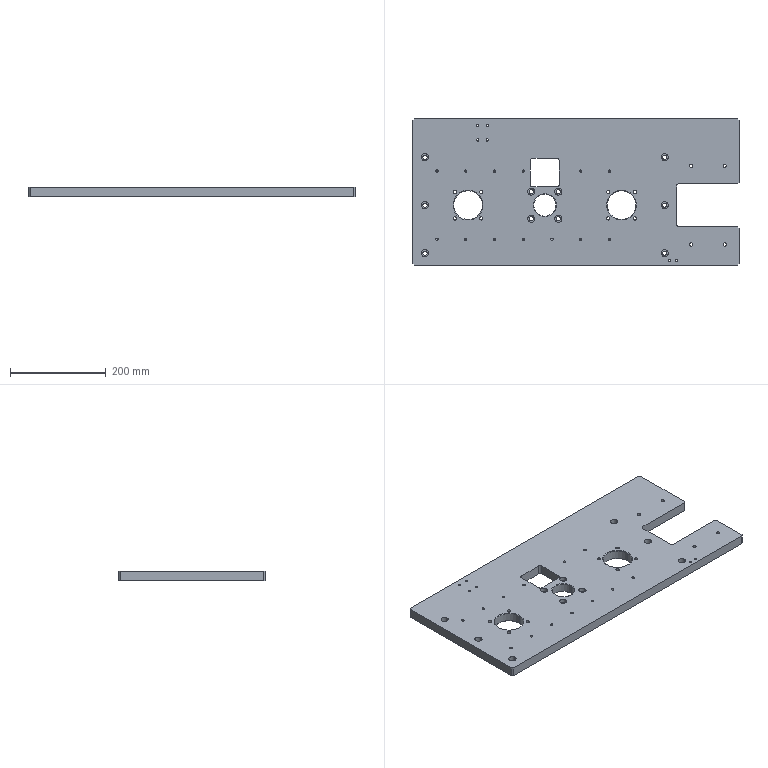Part | SolidWorks | features HoleWzd 7, Chamfer 2, Extrusion 1, Fillet 1, ICE 1 | 1 solid | 180 faces | box 680 x 305 x 20 mm | volume 3656558 mm3 | cylinder 114 | cone 36 | plane 30 | commonest cylinder face diameters 5 x38 6.8 x24 9 x20 15 x20 10 x6 60 x4